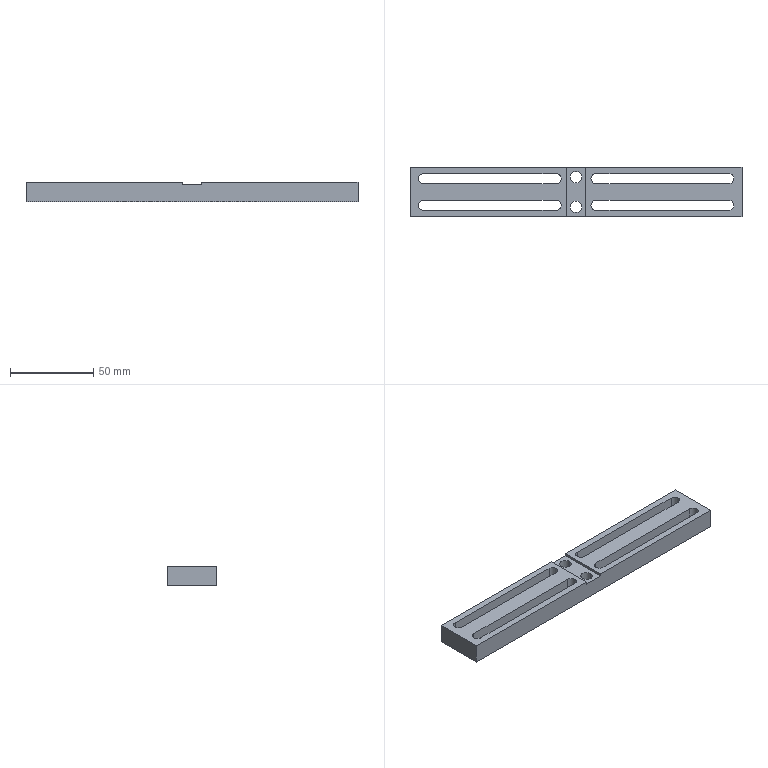Part | SolidWorks | features ICE 2, Extrusion 1 | 1 solid | 34 faces | box 200 x 30 x 12 mm | volume 46255 mm3 | plane 18 | cylinder 16 | commonest cylinder face diameters 6 x12 7 x4
STEP:
#1=CARTESIAN_POINT('',(-3.5,9.,0.));
#2=VERTEX_POINT('',#1);
#3=CARTESIAN_POINT('',(3.5,9.,0.));
#4=VERTEX_POINT('',#3);
#5=CARTESIAN_POINT('',(0.,9.,0.));
#6=DIRECTION('',(0.,0.,1.));
#7=DIRECTION('',(-1.,0.,0.));
#8=AXIS2_PLACEMENT_3D('',#5,#6,#7);
#9=CIRCLE('',#8,3.5);
#10=EDGE_CURVE('',#2,#4,#9,.T.);
#11=ORIENTED_EDGE('',*,*,#10,.F.);
#12=CARTESIAN_POINT('',(-3.5,9.,10.5));
#13=VERTEX_POINT('',#12);
#14=CARTESIAN_POINT('',(-3.5,9.,-0.001));
#15=DIRECTION('',(0.,0.,1.));
#16=VECTOR('',#15,1000.);
#17=LINE('',#14,#16);
#18=EDGE_CURVE('',#2,#13,#17,.T.);
#19=ORIENTED_EDGE('',*,*,#18,.T.);
#20=CARTESIAN_POINT('',(3.5,9.,10.5));
#21=VERTEX_POINT('',#20);
#22=CARTESIAN_POINT('',(0.,9.,10.5));
#23=DIRECTION('',(0.,0.,1.));
#24=DIRECTION('',(1.,0.,0.));
#25=AXIS2_PLACEMENT_3D('',#22,#23,#24);
#26=CIRCLE('',#25,3.5);
#27=EDGE_CURVE('',#13,#21,#26,.T.);
#28=ORIENTED_EDGE('',*,*,#27,.T.);
#29=CARTESIAN_POINT('',(3.5,9.,-0.001));
#30=DIRECTION('',(0.,0.,1.));
#31=VECTOR('',#30,1000.);
#32=LINE('',#29,#31);
#33=EDGE_CURVE('',#4,#21,#32,.T.);
#34=ORIENTED_EDGE('',*,*,#33,.F.);
#35=EDGE_LOOP('',(#11,#19,#28,#34));
#36=FACE_OUTER_BOUND('',#35,.T.);
#37=CARTESIAN_POINT('',(0.,9.,-0.001));
#38=DIRECTION('',(0.,0.,1.));
#39=DIRECTION('',(1.,0.,0.));
#40=AXIS2_PLACEMENT_3D('',#37,#38,#39);
#41=CYLINDRICAL_SURFACE('',#40,3.5);
#42=ADVANCED_FACE('',(#36),#41,.F.);
#43=CARTESIAN_POINT('',(-3.5,-9.,0.));
#44=VERTEX_POINT('',#43);
#45=CARTESIAN_POINT('',(3.5,-9.,0.));
#46=VERTEX_POINT('',#45);
#47=CARTESIAN_POINT('',(0.,-9.,0.));
#48=DIRECTION('',(0.,0.,1.));
#49=DIRECTION('',(-1.,0.,0.));
#50=AXIS2_PLACEMENT_3D('',#47,#48,#49);
#51=CIRCLE('',#50,3.5);
#52=EDGE_CURVE('',#44,#46,#51,.T.);
#53=ORIENTED_EDGE('',*,*,#52,.F.);
#54=CARTESIAN_POINT('',(-3.5,-9.,10.5));
#55=VERTEX_POINT('',#54);
#56=CARTESIAN_POINT('',(-3.5,-9.,-0.001));
#57=DIRECTION('',(0.,0.,1.));
#58=VECTOR('',#57,1000.);
#59=LINE('',#56,#58);
#60=EDGE_CURVE('',#44,#55,#59,.T.);
#61=ORIENTED_EDGE('',*,*,#60,.T.);
#62=CARTESIAN_POINT('',(3.5,-9.,10.5));
#63=VERTEX_POINT('',#62);
#64=CARTESIAN_POINT('',(0.,-9.,10.5));
#65=DIRECTION('',(0.,0.,1.));
#66=DIRECTION('',(1.,0.,0.));
#67=AXIS2_PLACEMENT_3D('',#64,#65,#66);
#68=CIRCLE('',#67,3.5);
#69=EDGE_CURVE('',#55,#63,#68,.T.);
#70=ORIENTED_EDGE('',*,*,#69,.T.);
#71=CARTESIAN_POINT('',(3.5,-9.,-0.001));
#72=DIRECTION('',(0.,0.,1.));
#73=VECTOR('',#72,1000.);
#74=LINE('',#71,#73);
#75=EDGE_CURVE('',#46,#63,#74,.T.);
#76=ORIENTED_EDGE('',*,*,#75,.F.);
#77=EDGE_LOOP('',(#53,#61,#70,#76));
#78=FACE_OUTER_BOUND('',#77,.T.);
#79=CARTESIAN_POINT('',(0.,-9.,-0.001));
#80=DIRECTION('',(0.,0.,1.));
#81=DIRECTION('',(1.,0.,0.));
#82=AXIS2_PLACEMENT_3D('',#79,#80,#81);
#83=CYLINDRICAL_SURFACE('',#82,3.5);
#84=ADVANCED_FACE('',(#78),#83,.F.);
#85=CARTESIAN_POINT('',(12.,-5.,12.));
#86=VERTEX_POINT('',#85);
#87=CARTESIAN_POINT('',(9.,-8.,12.));
#88=VERTEX_POINT('',#87);
#89=CARTESIAN_POINT('',(12.,-8.,12.));
#90=DIRECTION('',(0.,0.,1.));
#91=DIRECTION('',(1.,0.,0.));
#92=AXIS2_PLACEMENT_3D('',#89,#90,#91);
#93=CIRCLE('',#92,3.);
#94=EDGE_CURVE('',#86,#88,#93,.T.);
#95=ORIENTED_EDGE('',*,*,#94,.T.);
#96=CARTESIAN_POINT('',(9.,-8.,0.));
#97=VERTEX_POINT('',#96);
#98=CARTESIAN_POINT('',(9.,-8.,12.));
#99=DIRECTION('',(0.,0.,-1.));
#100=VECTOR('',#99,1000.);
#101=LINE('',#98,#100);
#102=EDGE_CURVE('',#88,#97,#101,.T.);
#103=ORIENTED_EDGE('',*,*,#102,.T.);
#104=CARTESIAN_POINT('',(12.,-5.,0.));
#105=VERTEX_POINT('',#104);
#106=CARTESIAN_POINT('',(12.,-8.,0.));
#107=DIRECTION('',(0.,0.,1.));
#108=DIRECTION('',(1.,0.,0.));
#109=AXIS2_PLACEMENT_3D('',#106,#107,#108);
#110=CIRCLE('',#109,3.);
#111=EDGE_CURVE('',#105,#97,#110,.T.);
#112=ORIENTED_EDGE('',*,*,#111,.F.);
#113=CARTESIAN_POINT('',(12.,-5.,12.));
#114=DIRECTION('',(0.,0.,-1.));
#115=VECTOR('',#114,1000.);
#116=LINE('',#113,#115);
#117=EDGE_CURVE('',#86,#105,#116,.T.);
#118=ORIENTED_EDGE('',*,*,#117,.F.);
#119=EDGE_LOOP('',(#95,#103,#112,#118));
#120=FACE_OUTER_BOUND('',#119,.T.);
#121=CARTESIAN_POINT('',(12.,-8.,12.));
#122=DIRECTION('',(0.,0.,-1.));
#123=DIRECTION('',(-1.,0.,0.));
#124=AXIS2_PLACEMENT_3D('',#121,#122,#123);
#125=CYLINDRICAL_SURFACE('',#124,3.);
#126=ADVANCED_FACE('',(#120),#125,.F.);
#127=CARTESIAN_POINT('',(12.,11.,12.));
#128=VERTEX_POINT('',#127);
#129=CARTESIAN_POINT('',(9.,8.,12.));
#130=VERTEX_POINT('',#129);
#131=CARTESIAN_POINT('',(12.,8.,12.));
#132=DIRECTION('',(0.,0.,1.));
#133=DIRECTION('',(-1.,0.,0.));
#134=AXIS2_PLACEMENT_3D('',#131,#132,#133);
#135=CIRCLE('',#134,3.);
#136=EDGE_CURVE('',#128,#130,#135,.T.);
#137=ORIENTED_EDGE('',*,*,#136,.T.);
#138=CARTESIAN_POINT('',(9.,8.,0.));
#139=VERTEX_POINT('',#138);
#140=CARTESIAN_POINT('',(9.,8.,12.));
#141=DIRECTION('',(0.,0.,-1.));
#142=VECTOR('',#141,1000.);
#143=LINE('',#140,#142);
#144=EDGE_CURVE('',#130,#139,#143,.T.);
#145=ORIENTED_EDGE('',*,*,#144,.T.);
#146=CARTESIAN_POINT('',(12.,11.,0.));
#147=VERTEX_POINT('',#146);
#148=CARTESIAN_POINT('',(12.,8.,0.));
#149=DIRECTION('',(0.,0.,1.));
#150=DIRECTION('',(-1.,0.,0.));
#151=AXIS2_PLACEMENT_3D('',#148,#149,#150);
#152=CIRCLE('',#151,3.);
#153=EDGE_CURVE('',#147,#139,#152,.T.);
#154=ORIENTED_EDGE('',*,*,#153,.F.);
#155=CARTESIAN_POINT('',(12.,11.,12.));
#156=DIRECTION('',(0.,0.,-1.));
#157=VECTOR('',#156,1000.);
#158=LINE('',#155,#157);
#159=EDGE_CURVE('',#128,#147,#158,.T.);
#160=ORIENTED_EDGE('',*,*,#159,.F.);
#161=EDGE_LOOP('',(#137,#145,#154,#160));
#162=FACE_OUTER_BOUND('',#161,.T.);
#163=CARTESIAN_POINT('',(12.,8.,12.));
#164=DIRECTION('',(0.,0.,-1.));
#165=DIRECTION('',(-1.,0.,0.));
#166=AXIS2_PLACEMENT_3D('',#163,#164,#165);
#167=CYLINDRICAL_SURFACE('',#166,3.);
#168=ADVANCED_FACE('',(#162),#167,.F.);
#169=CARTESIAN_POINT('',(-92.,-5.,12.));
#170=VERTEX_POINT('',#169);
#171=CARTESIAN_POINT('',(-95.,-8.,12.));
#172=VERTEX_POINT('',#171);
#173=CARTESIAN_POINT('',(-92.,-8.,12.));
#174=DIRECTION('',(0.,0.,1.));
#175=DIRECTION('',(-1.,0.,0.));
#176=AXIS2_PLACEMENT_3D('',#173,#174,#175);
#177=CIRCLE('',#176,3.);
#178=EDGE_CURVE('',#170,#172,#177,.T.);
#179=ORIENTED_EDGE('',*,*,#178,.T.);
#180=CARTESIAN_POINT('',(-95.,-8.,0.));
#181=VERTEX_POINT('',#180);
#182=CARTESIAN_POINT('',(-95.,-8.,12.));
#183=DIRECTION('',(0.,0.,-1.));
#184=VECTOR('',#183,1000.);
#185=LINE('',#182,#184);
#186=EDGE_CURVE('',#172,#181,#185,.T.);
#187=ORIENTED_EDGE('',*,*,#186,.T.);
#188=CARTESIAN_POINT('',(-92.,-5.,0.));
#189=VERTEX_POINT('',#188);
#190=CARTESIAN_POINT('',(-92.,-8.,0.));
#191=DIRECTION('',(0.,0.,1.));
#192=DIRECTION('',(-1.,0.,0.));
#193=AXIS2_PLACEMENT_3D('',#190,#191,#192);
#194=CIRCLE('',#193,3.);
#195=EDGE_CURVE('',#189,#181,#194,.T.);
#196=ORIENTED_EDGE('',*,*,#195,.F.);
#197=CARTESIAN_POINT('',(-92.,-5.,12.));
#198=DIRECTION('',(0.,0.,-1.));
#199=VECTOR('',#198,1000.);
#200=LINE('',#197,#199);
#201=EDGE_CURVE('',#170,#189,#200,.T.);
#202=ORIENTED_EDGE('',*,*,#201,.F.);
#203=EDGE_LOOP('',(#179,#187,#196,#202));
#204=FACE_OUTER_BOUND('',#203,.T.);
#205=CARTESIAN_POINT('',(-92.,-8.,12.));
#206=DIRECTION('',(0.,0.,-1.));
#207=DIRECTION('',(-1.,0.,0.));
#208=AXIS2_PLACEMENT_3D('',#205,#206,#207);
#209=CYLINDRICAL_SURFACE('',#208,3.);
#210=ADVANCED_FACE('',(#204),#209,.F.);
#211=CARTESIAN_POINT('',(-92.,11.,12.));
#212=VERTEX_POINT('',#211);
#213=CARTESIAN_POINT('',(-95.,8.,12.));
#214=VERTEX_POINT('',#213);
#215=CARTESIAN_POINT('',(-92.,8.,12.));
#216=DIRECTION('',(0.,0.,1.));
#217=DIRECTION('',(1.,0.,0.));
#218=AXIS2_PLACEMENT_3D('',#215,#216,#217);
#219=CIRCLE('',#218,3.);
#220=EDGE_CURVE('',#212,#214,#219,.T.);
#221=ORIENTED_EDGE('',*,*,#220,.T.);
#222=CARTESIAN_POINT('',(-95.,8.,0.));
#223=VERTEX_POINT('',#222);
#224=CARTESIAN_POINT('',(-95.,8.,12.));
#225=DIRECTION('',(0.,0.,-1.));
#226=VECTOR('',#225,1000.);
#227=LINE('',#224,#226);
#228=EDGE_CURVE('',#214,#223,#227,.T.);
#229=ORIENTED_EDGE('',*,*,#228,.T.);
#230=CARTESIAN_POINT('',(-92.,11.,0.));
#231=VERTEX_POINT('',#230);
#232=CARTESIAN_POINT('',(-92.,8.,0.));
#233=DIRECTION('',(0.,0.,1.));
#234=DIRECTION('',(1.,0.,0.));
#235=AXIS2_PLACEMENT_3D('',#232,#233,#234);
#236=CIRCLE('',#235,3.);
#237=EDGE_CURVE('',#231,#223,#236,.T.);
#238=ORIENTED_EDGE('',*,*,#237,.F.);
#239=CARTESIAN_POINT('',(-92.,11.,12.));
#240=DIRECTION('',(0.,0.,-1.));
#241=VECTOR('',#240,1000.);
#242=LINE('',#239,#241);
#243=EDGE_CURVE('',#212,#231,#242,.T.);
#244=ORIENTED_EDGE('',*,*,#243,.F.);
#245=EDGE_LOOP('',(#221,#229,#238,#244));
#246=FACE_OUTER_BOUND('',#245,.T.);
#247=CARTESIAN_POINT('',(-92.,8.,12.));
#248=DIRECTION('',(0.,0.,-1.));
#249=DIRECTION('',(-1.,0.,0.));
#250=AXIS2_PLACEMENT_3D('',#247,#248,#249);
#251=CYLINDRICAL_SURFACE('',#250,3.);
#252=ADVANCED_FACE('',(#246),#251,.F.);
#253=CARTESIAN_POINT('',(92.,-11.,12.));
#254=VERTEX_POINT('',#253);
#255=CARTESIAN_POINT('',(92.,-5.,12.));
#256=VERTEX_POINT('',#255);
#257=CARTESIAN_POINT('',(92.,-8.,12.));
#258=DIRECTION('',(0.,0.,1.));
#259=DIRECTION('',(1.,0.,0.));
#260=AXIS2_PLACEMENT_3D('',#257,#258,#259);
#261=CIRCLE('',#260,3.);
#262=EDGE_CURVE('',#254,#256,#261,.T.);
#263=ORIENTED_EDGE('',*,*,#262,.F.);
#264=CARTESIAN_POINT('',(12.,-11.,12.));
#265=VERTEX_POINT('',#264);
#266=CARTESIAN_POINT('',(92.,-11.,12.));
#267=DIRECTION('',(1.,0.,0.));
#268=VECTOR('',#267,1000.);
#269=LINE('',#266,#268);
#270=EDGE_CURVE('',#265,#254,#269,.T.);
#271=ORIENTED_EDGE('',*,*,#270,.F.);
#272=CARTESIAN_POINT('',(12.,-8.,12.));
#273=DIRECTION('',(0.,0.,1.));
#274=DIRECTION('',(1.,0.,0.));
#275=AXIS2_PLACEMENT_3D('',#272,#273,#274);
#276=CIRCLE('',#275,3.);
#277=EDGE_CURVE('',#88,#265,#276,.T.);
#278=ORIENTED_EDGE('',*,*,#277,.F.);
#279=ORIENTED_EDGE('',*,*,#94,.F.);
#280=CARTESIAN_POINT('',(92.,-5.,12.));
#281=DIRECTION('',(-1.,0.,0.));
#282=VECTOR('',#281,1000.);
#283=LINE('',#280,#282);
#284=EDGE_CURVE('',#256,#86,#283,.T.);
#285=ORIENTED_EDGE('',*,*,#284,.F.);
#286=EDGE_LOOP('',(#263,#271,#278,#279,#285));
#287=FACE_BOUND('',#286,.T.);
#288=CARTESIAN_POINT('',(92.,5.,12.));
#289=VERTEX_POINT('',#288);
#290=CARTESIAN_POINT('',(92.,11.,12.));
#291=VERTEX_POINT('',#290);
#292=CARTESIAN_POINT('',(92.,8.,12.));
#293=DIRECTION('',(0.,0.,1.));
#294=DIRECTION('',(-1.,0.,0.));
#295=AXIS2_PLACEMENT_3D('',#292,#293,#294);
#296=CIRCLE('',#295,3.);
#297=EDGE_CURVE('',#289,#291,#296,.T.);
#298=ORIENTED_EDGE('',*,*,#297,.F.);
#299=CARTESIAN_POINT('',(12.,5.,12.));
#300=VERTEX_POINT('',#299);
#301=CARTESIAN_POINT('',(92.,5.,12.));
#302=DIRECTION('',(1.,0.,0.));
#303=VECTOR('',#302,1000.);
#304=LINE('',#301,#303);
#305=EDGE_CURVE('',#300,#289,#304,.T.);
#306=ORIENTED_EDGE('',*,*,#305,.F.);
#307=CARTESIAN_POINT('',(12.,8.,12.));
#308=DIRECTION('',(0.,0.,1.));
#309=DIRECTION('',(-1.,0.,0.));
#310=AXIS2_PLACEMENT_3D('',#307,#308,#309);
#311=CIRCLE('',#310,3.);
#312=EDGE_CURVE('',#130,#300,#311,.T.);
#313=ORIENTED_EDGE('',*,*,#312,.F.);
#314=ORIENTED_EDGE('',*,*,#136,.F.);
#315=CARTESIAN_POINT('',(92.,11.,12.));
#316=DIRECTION('',(-1.,0.,0.));
#317=VECTOR('',#316,1000.);
#318=LINE('',#315,#317);
#319=EDGE_CURVE('',#291,#128,#318,.T.);
#320=ORIENTED_EDGE('',*,*,#319,.F.);
#321=EDGE_LOOP('',(#298,#306,#313,#314,#320));
#322=FACE_BOUND('',#321,.T.);
#323=CARTESIAN_POINT('',(100.,15.,12.));
#324=VERTEX_POINT('',#323);
#325=CARTESIAN_POINT('',(6.,15.,12.));
#326=VERTEX_POINT('',#325);
#327=CARTESIAN_POINT('',(-100.,15.,12.));
#328=DIRECTION('',(-1.,0.,0.));
#329=VECTOR('',#328,1000.);
#330=LINE('',#327,#329);
#331=EDGE_CURVE('',#324,#326,#330,.T.);
#332=ORIENTED_EDGE('',*,*,#331,.T.);
#333=CARTESIAN_POINT('',(6.,-15.,12.));
#334=VERTEX_POINT('',#333);
#335=CARTESIAN_POINT('',(6.,-15.,12.));
#336=DIRECTION('',(0.,1.,0.));
#337=VECTOR('',#336,1000.);
#338=LINE('',#335,#337);
#339=EDGE_CURVE('',#334,#326,#338,.T.);
#340=ORIENTED_EDGE('',*,*,#339,.F.);
#341=CARTESIAN_POINT('',(100.,-15.,12.));
#342=VERTEX_POINT('',#341);
#343=CARTESIAN_POINT('',(-100.,-15.,12.));
#344=DIRECTION('',(1.,0.,0.));
#345=VECTOR('',#344,1000.);
#346=LINE('',#343,#345);
#347=EDGE_CURVE('',#334,#342,#346,.T.);
#348=ORIENTED_EDGE('',*,*,#347,.T.);
#349=CARTESIAN_POINT('',(100.,-15.,12.));
#350=DIRECTION('',(0.,1.,0.));
#351=VECTOR('',#350,1000.);
#352=LINE('',#349,#351);
#353=EDGE_CURVE('',#342,#324,#352,.T.);
#354=ORIENTED_EDGE('',*,*,#353,.T.);
#355=EDGE_LOOP('',(#332,#340,#348,#354));
#356=FACE_OUTER_BOUND('',#355,.T.);
#357=CARTESIAN_POINT('',(0.,0.,12.));
#358=DIRECTION('',(0.,0.,-1.));
#359=DIRECTION('',(-1.,0.,0.));
#360=AXIS2_PLACEMENT_3D('',#357,#358,#359);
#361=PLANE('',#360);
#362=ADVANCED_FACE('',(#287,#322,#356),#361,.F.);
#363=ORIENTED_EDGE('',*,*,#220,.F.);
#364=CARTESIAN_POINT('',(-12.,11.,12.));
#365=VERTEX_POINT('',#364);
#366=CARTESIAN_POINT('',(-92.,11.,12.));
#367=DIRECTION('',(-1.,0.,0.));
#368=VECTOR('',#367,1000.);
#369=LINE('',#366,#368);
#370=EDGE_CURVE('',#365,#212,#369,.T.);
#371=ORIENTED_EDGE('',*,*,#370,.F.);
#372=CARTESIAN_POINT('',(-12.,5.,12.));
#373=VERTEX_POINT('',#372);
#374=CARTESIAN_POINT('',(-12.,8.,12.));
#375=DIRECTION('',(0.,0.,1.));
#376=DIRECTION('',(1.,0.,0.));
#377=AXIS2_PLACEMENT_3D('',#374,#375,#376);
#378=CIRCLE('',#377,3.);
#379=EDGE_CURVE('',#373,#365,#378,.T.);
#380=ORIENTED_EDGE('',*,*,#379,.F.);
#381=CARTESIAN_POINT('',(-92.,5.,12.));
#382=VERTEX_POINT('',#381);
#383=CARTESIAN_POINT('',(-92.,5.,12.));
#384=DIRECTION('',(1.,0.,0.));
#385=VECTOR('',#384,1000.);
#386=LINE('',#383,#385);
#387=EDGE_CURVE('',#382,#373,#386,.T.);
#388=ORIENTED_EDGE('',*,*,#387,.F.);
#389=CARTESIAN_POINT('',(-92.,8.,12.));
#390=DIRECTION('',(0.,0.,1.));
#391=DIRECTION('',(1.,0.,0.));
#392=AXIS2_PLACEMENT_3D('',#389,#390,#391);
#393=CIRCLE('',#392,3.);
#394=EDGE_CURVE('',#214,#382,#393,.T.);
#395=ORIENTED_EDGE('',*,*,#394,.F.);
#396=EDGE_LOOP('',(#363,#371,#380,#388,#395));
#397=FACE_BOUND('',#396,.T.);
#398=CARTESIAN_POINT('',(-100.,-15.,12.));
#399=VERTEX_POINT('',#398);
#400=CARTESIAN_POINT('',(-6.,-15.,12.));
#401=VERTEX_POINT('',#400);
#402=CARTESIAN_POINT('',(-100.,-15.,12.));
#403=DIRECTION('',(1.,0.,0.));
#404=VECTOR('',#403,1000.);
#405=LINE('',#402,#404);
#406=EDGE_CURVE('',#399,#401,#405,.T.);
#407=ORIENTED_EDGE('',*,*,#406,.T.);
#408=CARTESIAN_POINT('',(-6.,15.,12.));
#409=VERTEX_POINT('',#408);
#410=CARTESIAN_POINT('',(-6.,-15.,12.));
#411=DIRECTION('',(0.,-1.,0.));
#412=VECTOR('',#411,1000.);
#413=LINE('',#410,#412);
#414=EDGE_CURVE('',#409,#401,#413,.T.);
#415=ORIENTED_EDGE('',*,*,#414,.F.);
#416=CARTESIAN_POINT('',(-100.,15.,12.));
#417=VERTEX_POINT('',#416);
#418=CARTESIAN_POINT('',(-100.,15.,12.));
#419=DIRECTION('',(-1.,0.,0.));
#420=VECTOR('',#419,1000.);
#421=LINE('',#418,#420);
#422=EDGE_CURVE('',#409,#417,#421,.T.);
#423=ORIENTED_EDGE('',*,*,#422,.T.);
#424=CARTESIAN_POINT('',(-100.,-15.,12.));
#425=DIRECTION('',(0.,-1.,0.));
#426=VECTOR('',#425,1000.);
#427=LINE('',#424,#426);
#428=EDGE_CURVE('',#417,#399,#427,.T.);
#429=ORIENTED_EDGE('',*,*,#428,.T.);
#430=EDGE_LOOP('',(#407,#415,#423,#429));
#431=FACE_OUTER_BOUND('',#430,.T.);
#432=ORIENTED_EDGE('',*,*,#178,.F.);
#433=CARTESIAN_POINT('',(-12.,-5.,12.));
#434=VERTEX_POINT('',#433);
#435=CARTESIAN_POINT('',(-92.,-5.,12.));
#436=DIRECTION('',(-1.,0.,0.));
#437=VECTOR('',#436,1000.);
#438=LINE('',#435,#437);
#439=EDGE_CURVE('',#434,#170,#438,.T.);
#440=ORIENTED_EDGE('',*,*,#439,.F.);
#441=CARTESIAN_POINT('',(-12.,-11.,12.));
#442=VERTEX_POINT('',#441);
#443=CARTESIAN_POINT('',(-12.,-8.,12.));
#444=DIRECTION('',(0.,0.,1.));
#445=DIRECTION('',(-1.,0.,0.));
#446=AXIS2_PLACEMENT_3D('',#443,#444,#445);
#447=CIRCLE('',#446,3.);
#448=EDGE_CURVE('',#442,#434,#447,.T.);
#449=ORIENTED_EDGE('',*,*,#448,.F.);
#450=CARTESIAN_POINT('',(-92.,-11.,12.));
#451=VERTEX_POINT('',#450);
#452=CARTESIAN_POINT('',(-92.,-11.,12.));
#453=DIRECTION('',(1.,0.,0.));
#454=VECTOR('',#453,1000.);
#455=LINE('',#452,#454);
#456=EDGE_CURVE('',#451,#442,#455,.T.);
#457=ORIENTED_EDGE('',*,*,#456,.F.);
#458=CARTESIAN_POINT('',(-92.,-8.,12.));
#459=DIRECTION('',(0.,0.,1.));
#460=DIRECTION('',(-1.,0.,0.));
#461=AXIS2_PLACEMENT_3D('',#458,#459,#460);
#462=CIRCLE('',#461,3.);
#463=EDGE_CURVE('',#172,#451,#462,.T.);
#464=ORIENTED_EDGE('',*,*,#463,.F.);
#465=EDGE_LOOP('',(#432,#440,#449,#457,#464));
#466=FACE_BOUND('',#465,.T.);
#467=CARTESIAN_POINT('',(0.,0.,12.));
#468=DIRECTION('',(0.,0.,-1.));
#469=DIRECTION('',(-1.,0.,0.));
#470=AXIS2_PLACEMENT_3D('',#467,#468,#469);
#471=PLANE('',#470);
#472=ADVANCED_FACE('',(#397,#431,#466),#471,.F.);
#473=CARTESIAN_POINT('',(0.,9.,0.));
#474=DIRECTION('',(0.,0.,1.));
#475=DIRECTION('',(-1.,0.,0.));
#476=AXIS2_PLACEMENT_3D('',#473,#474,#475);
#477=CIRCLE('',#476,3.5);
#478=EDGE_CURVE('',#4,#2,#477,.T.);
#479=ORIENTED_EDGE('',*,*,#478,.T.);
#480=ORIENTED_EDGE('',*,*,#10,.T.);
#481=EDGE_LOOP('',(#479,#480));
#482=FACE_BOUND('',#481,.T.);
#483=CARTESIAN_POINT('',(0.,-9.,0.));
#484=DIRECTION('',(0.,0.,1.));
#485=DIRECTION('',(-1.,0.,0.));
#486=AXIS2_PLACEMENT_3D('',#483,#484,#485);
#487=CIRCLE('',#486,3.5);
#488=EDGE_CURVE('',#46,#44,#487,.T.);
#489=ORIENTED_EDGE('',*,*,#488,.T.);
#490=ORIENTED_EDGE('',*,*,#52,.T.);
#491=EDGE_LOOP('',(#489,#490));
#492=FACE_BOUND('',#491,.T.);
#493=CARTESIAN_POINT('',(100.,-15.,0.));
#494=VERTEX_POINT('',#493);
#495=CARTESIAN_POINT('',(100.,15.,0.));
#496=VERTEX_POINT('',#495);
#497=CARTESIAN_POINT('',(100.,-15.,0.));
#498=DIRECTION('',(0.,1.,0.));
#499=VECTOR('',#498,1000.);
#500=LINE('',#497,#499);
#501=EDGE_CURVE('',#494,#496,#500,.T.);
#502=ORIENTED_EDGE('',*,*,#501,.F.);
#503=CARTESIAN_POINT('',(-100.,-15.,0.));
#504=VERTEX_POINT('',#503);
#505=CARTESIAN_POINT('',(-100.,-15.,0.));
#506=DIRECTION('',(1.,0.,0.));
#507=VECTOR('',#506,1000.);
#508=LINE('',#505,#507);
#509=EDGE_CURVE('',#504,#494,#508,.T.);
#510=ORIENTED_EDGE('',*,*,#509,.F.);
#511=CARTESIAN_POINT('',(-100.,15.,0.));
#512=VERTEX_POINT('',#511);
#513=CARTESIAN_POINT('',(-100.,-15.,0.));
#514=DIRECTION('',(0.,-1.,0.));
#515=VECTOR('',#514,1000.);
#516=LINE('',#513,#515);
#517=EDGE_CURVE('',#512,#504,#516,.T.);
#518=ORIENTED_EDGE('',*,*,#517,.F.);
#519=CARTESIAN_POINT('',(-100.,15.,0.));
#520=DIRECTION('',(-1.,0.,0.));
#521=VECTOR('',#520,1000.);
#522=LINE('',#519,#521);
#523=EDGE_CURVE('',#496,#512,#522,.T.);
#524=ORIENTED_EDGE('',*,*,#523,.F.);
#525=EDGE_LOOP('',(#502,#510,#518,#524));
#526=FACE_OUTER_BOUND('',#525,.T.);
#527=CARTESIAN_POINT('',(-12.,11.,0.));
#528=VERTEX_POINT('',#527);
#529=CARTESIAN_POINT('',(-92.,11.,0.));
#530=DIRECTION('',(-1.,0.,0.));
#531=VECTOR('',#530,1000.);
#532=LINE('',#529,#531);
#533=EDGE_CURVE('',#528,#231,#532,.T.);
#534=ORIENTED_EDGE('',*,*,#533,.T.);
#535=ORIENTED_EDGE('',*,*,#237,.T.);
#536=CARTESIAN_POINT('',(-92.,5.,0.));
#537=VERTEX_POINT('',#536);
#538=CARTESIAN_POINT('',(-92.,8.,0.));
#539=DIRECTION('',(0.,0.,1.));
#540=DIRECTION('',(1.,0.,0.));
#541=AXIS2_PLACEMENT_3D('',#538,#539,#540);
#542=CIRCLE('',#541,3.);
#543=EDGE_CURVE('',#223,#537,#542,.T.);
#544=ORIENTED_EDGE('',*,*,#543,.T.);
#545=CARTESIAN_POINT('',(-12.,5.,0.));
#546=VERTEX_POINT('',#545);
#547=CARTESIAN_POINT('',(-92.,5.,0.));
#548=DIRECTION('',(1.,0.,0.));
#549=VECTOR('',#548,1000.);
#550=LINE('',#547,#549);
#551=EDGE_CURVE('',#537,#546,#550,.T.);
#552=ORIENTED_EDGE('',*,*,#551,.T.);
#553=CARTESIAN_POINT('',(-12.,8.,0.));
#554=DIRECTION('',(0.,0.,1.));
#555=DIRECTION('',(1.,0.,0.));
#556=AXIS2_PLACEMENT_3D('',#553,#554,#555);
#557=CIRCLE('',#556,3.);
#558=EDGE_CURVE('',#546,#528,#557,.T.);
#559=ORIENTED_EDGE('',*,*,#558,.T.);
#560=EDGE_LOOP('',(#534,#535,#544,#552,#559));
#561=FACE_BOUND('',#560,.T.);
#562=CARTESIAN_POINT('',(-12.,-5.,0.));
#563=VERTEX_POINT('',#562);
#564=CARTESIAN_POINT('',(-92.,-5.,0.));
#565=DIRECTION('',(-1.,0.,0.));
#566=VECTOR('',#565,1000.);
#567=LINE('',#564,#566);
#568=EDGE_CURVE('',#563,#189,#567,.T.);
#569=ORIENTED_EDGE('',*,*,#568,.T.);
#570=ORIENTED_EDGE('',*,*,#195,.T.);
#571=CARTESIAN_POINT('',(-92.,-11.,0.));
#572=VERTEX_POINT('',#571);
#573=CARTESIAN_POINT('',(-92.,-8.,0.));
#574=DIRECTION('',(0.,0.,1.));
#575=DIRECTION('',(-1.,0.,0.));
#576=AXIS2_PLACEMENT_3D('',#573,#574,#575);
#577=CIRCLE('',#576,3.);
#578=EDGE_CURVE('',#181,#572,#577,.T.);
#579=ORIENTED_EDGE('',*,*,#578,.T.);
#580=CARTESIAN_POINT('',(-12.,-11.,0.));
#581=VERTEX_POINT('',#580);
#582=CARTESIAN_POINT('',(-92.,-11.,0.));
#583=DIRECTION('',(1.,0.,0.));
#584=VECTOR('',#583,1000.);
#585=LINE('',#582,#584);
#586=EDGE_CURVE('',#572,#581,#585,.T.);
#587=ORIENTED_EDGE('',*,*,#586,.T.);
#588=CARTESIAN_POINT('',(-12.,-8.,0.));
#589=DIRECTION('',(0.,0.,1.));
#590=DIRECTION('',(-1.,0.,0.));
#591=AXIS2_PLACEMENT_3D('',#588,#589,#590);
#592=CIRCLE('',#591,3.);
#593=EDGE_CURVE('',#581,#563,#592,.T.);
#594=ORIENTED_EDGE('',*,*,#593,.T.);
#595=EDGE_LOOP('',(#569,#570,#579,#587,#594));
#596=FACE_BOUND('',#595,.T.);
#597=CARTESIAN_POINT('',(12.,5.,0.));
#598=VERTEX_POINT('',#597);
#599=CARTESIAN_POINT('',(92.,5.,0.));
#600=VERTEX_POINT('',#599);
#601=CARTESIAN_POINT('',(92.,5.,0.));
#602=DIRECTION('',(1.,0.,0.));
#603=VECTOR('',#602,1000.);
#604=LINE('',#601,#603);
#605=EDGE_CURVE('',#598,#600,#604,.T.);
#606=ORIENTED_EDGE('',*,*,#605,.T.);
#607=CARTESIAN_POINT('',(92.,11.,0.));
#608=VERTEX_POINT('',#607);
#609=CARTESIAN_POINT('',(92.,8.,0.));
#610=DIRECTION('',(0.,0.,1.));
#611=DIRECTION('',(-1.,0.,0.));
#612=AXIS2_PLACEMENT_3D('',#609,#610,#611);
#613=CIRCLE('',#612,3.);
#614=EDGE_CURVE('',#600,#608,#613,.T.);
#615=ORIENTED_EDGE('',*,*,#614,.T.);
#616=CARTESIAN_POINT('',(92.,11.,0.));
#617=DIRECTION('',(-1.,0.,0.));
#618=VECTOR('',#617,1000.);
#619=LINE('',#616,#618);
#620=EDGE_CURVE('',#608,#147,#619,.T.);
#621=ORIENTED_EDGE('',*,*,#620,.T.);
#622=ORIENTED_EDGE('',*,*,#153,.T.);
#623=CARTESIAN_POINT('',(12.,8.,0.));
#624=DIRECTION('',(0.,0.,1.));
#625=DIRECTION('',(-1.,0.,0.));
#626=AXIS2_PLACEMENT_3D('',#623,#624,#625);
#627=CIRCLE('',#626,3.);
#628=EDGE_CURVE('',#139,#598,#627,.T.);
#629=ORIENTED_EDGE('',*,*,#628,.T.);
#630=EDGE_LOOP('',(#606,#615,#621,#622,#629));
#631=FACE_BOUND('',#630,.T.);
#632=CARTESIAN_POINT('',(12.,-11.,0.));
#633=VERTEX_POINT('',#632);
#634=CARTESIAN_POINT('',(92.,-11.,0.));
#635=VERTEX_POINT('',#634);
#636=CARTESIAN_POINT('',(92.,-11.,0.));
#637=DIRECTION('',(1.,0.,0.));
#638=VECTOR('',#637,1000.);
#639=LINE('',#636,#638);
#640=EDGE_CURVE('',#633,#635,#639,.T.);
#641=ORIENTED_EDGE('',*,*,#640,.T.);
#642=CARTESIAN_POINT('',(92.,-5.,0.));
#643=VERTEX_POINT('',#642);
#644=CARTESIAN_POINT('',(92.,-8.,0.));
#645=DIRECTION('',(0.,0.,1.));
#646=DIRECTION('',(1.,0.,0.));
#647=AXIS2_PLACEMENT_3D('',#644,#645,#646);
#648=CIRCLE('',#647,3.);
#649=EDGE_CURVE('',#635,#643,#648,.T.);
#650=ORIENTED_EDGE('',*,*,#649,.T.);
#651=CARTESIAN_POINT('',(92.,-5.,0.));
#652=DIRECTION('',(-1.,0.,0.));
#653=VECTOR('',#652,1000.);
#654=LINE('',#651,#653);
#655=EDGE_CURVE('',#643,#105,#654,.T.);
#656=ORIENTED_EDGE('',*,*,#655,.T.);
#657=ORIENTED_EDGE('',*,*,#111,.T.);
#658=CARTESIAN_POINT('',(12.,-8.,0.));
#659=DIRECTION('',(0.,0.,1.));
#660=DIRECTION('',(1.,0.,0.));
#661=AXIS2_PLACEMENT_3D('',#658,#659,#660);
#662=CIRCLE('',#661,3.);
#663=EDGE_CURVE('',#97,#633,#662,.T.);
#664=ORIENTED_EDGE('',*,*,#663,.T.);
#665=EDGE_LOOP('',(#641,#650,#656,#657,#664));
#666=FACE_BOUND('',#665,.T.);
#667=CARTESIAN_POINT('',(0.,0.,0.));
#668=DIRECTION('',(0.,0.,-1.));
#669=DIRECTION('',(-1.,0.,0.));
#670=AXIS2_PLACEMENT_3D('',#667,#668,#669);
#671=PLANE('',#670);
#672=ADVANCED_FACE('',(#482,#492,#526,#561,#596,#631,#666),#671,.T.);
#673=ORIENTED_EDGE('',*,*,#501,.T.);
#674=CARTESIAN_POINT('',(100.,15.,12.));
#675=DIRECTION('',(0.,0.,-1.));
#676=VECTOR('',#675,1000.);
#677=LINE('',#674,#676);
#678=EDGE_CURVE('',#324,#496,#677,.T.);
#679=ORIENTED_EDGE('',*,*,#678,.F.);
#680=ORIENTED_EDGE('',*,*,#353,.F.);
#681=CARTESIAN_POINT('',(100.,-15.,12.));
#682=DIRECTION('',(0.,0.,-1.));
#683=VECTOR('',#682,1000.);
#684=LINE('',#681,#683);
#685=EDGE_CURVE('',#342,#494,#684,.T.);
#686=ORIENTED_EDGE('',*,*,#685,.T.);
#687=EDGE_LOOP('',(#673,#679,#680,#686));
#688=FACE_OUTER_BOUND('',#687,.T.);
#689=CARTESIAN_POINT('',(100.,-15.,12.));
#690=DIRECTION('',(-1.,0.,0.));
#691=DIRECTION('',(0.,0.,1.));
#692=AXIS2_PLACEMENT_3D('',#689,#690,#691);
#693=PLANE('',#692);
#694=ADVANCED_FACE('',(#688),#693,.F.);
#695=CARTESIAN_POINT('',(6.,15.,10.5));
#696=VERTEX_POINT('',#695);
#697=CARTESIAN_POINT('',(-6.,15.,10.5));
#698=VERTEX_POINT('',#697);
#699=CARTESIAN_POINT('',(-6.,15.,10.5));
#700=DIRECTION('',(-1.,0.,0.));
#701=VECTOR('',#700,1000.);
#702=LINE('',#699,#701);
#703=EDGE_CURVE('',#696,#698,#702,.T.);
#704=ORIENTED_EDGE('',*,*,#703,.F.);
#705=CARTESIAN_POINT('',(6.,15.,10.5));
#706=DIRECTION('',(0.,0.,1.));
#707=VECTOR('',#706,1000.);
#708=LINE('',#705,#707);
#709=EDGE_CURVE('',#696,#326,#708,.T.);
#710=ORIENTED_EDGE('',*,*,#709,.T.);
#711=ORIENTED_EDGE('',*,*,#331,.F.);
#712=ORIENTED_EDGE('',*,*,#678,.T.);
#713=ORIENTED_EDGE('',*,*,#523,.T.);
#714=CARTESIAN_POINT('',(-100.,15.,12.));
#715=DIRECTION('',(0.,0.,-1.));
#716=VECTOR('',#715,1000.);
#717=LINE('',#714,#716);
#718=EDGE_CURVE('',#417,#512,#717,.T.);
#719=ORIENTED_EDGE('',*,*,#718,.F.);
#720=ORIENTED_EDGE('',*,*,#422,.F.);
#721=CARTESIAN_POINT('',(-6.,15.,10.5));
#722=DIRECTION('',(0.,0.,1.));
#723=VECTOR('',#722,1000.);
#724=LINE('',#721,#723);
#725=EDGE_CURVE('',#698,#409,#724,.T.);
#726=ORIENTED_EDGE('',*,*,#725,.F.);
#727=EDGE_LOOP('',(#704,#710,#711,#712,#713,#719,#720,#726));
#728=FACE_OUTER_BOUND('',#727,.T.);
#729=CARTESIAN_POINT('',(-100.,15.,12.));
#730=DIRECTION('',(0.,-1.,0.));
#731=DIRECTION('',(0.,0.,-1.));
#732=AXIS2_PLACEMENT_3D('',#729,#730,#731);
#733=PLANE('',#732);
#734=ADVANCED_FACE('',(#728),#733,.F.);
#735=ORIENTED_EDGE('',*,*,#517,.T.);
#736=CARTESIAN_POINT('',(-100.,-15.,12.));
#737=DIRECTION('',(0.,0.,-1.));
#738=VECTOR('',#737,1000.);
#739=LINE('',#736,#738);
#740=EDGE_CURVE('',#399,#504,#739,.T.);
#741=ORIENTED_EDGE('',*,*,#740,.F.);
#742=ORIENTED_EDGE('',*,*,#428,.F.);
#743=ORIENTED_EDGE('',*,*,#718,.T.);
#744=EDGE_LOOP('',(#735,#741,#742,#743));
#745=FACE_OUTER_BOUND('',#744,.T.);
#746=CARTESIAN_POINT('',(-100.,-15.,12.));
#747=DIRECTION('',(1.,0.,0.));
#748=DIRECTION('',(0.,0.,-1.));
#749=AXIS2_PLACEMENT_3D('',#746,#747,#748);
#750=PLANE('',#749);
#751=ADVANCED_FACE('',(#745),#750,.F.);
#752=ORIENTED_EDGE('',*,*,#347,.F.);
#753=CARTESIAN_POINT('',(6.,-15.,10.5));
#754=VERTEX_POINT('',#753);
#755=CARTESIAN_POINT('',(6.,-15.,10.5));
#756=DIRECTION('',(0.,0.,1.));
#757=VECTOR('',#756,1000.);
#758=LINE('',#755,#757);
#759=EDGE_CURVE('',#754,#334,#758,.T.);
#760=ORIENTED_EDGE('',*,*,#759,.F.);
#761=CARTESIAN_POINT('',(-6.,-15.,10.5));
#762=VERTEX_POINT('',#761);
#763=CARTESIAN_POINT('',(-6.,-15.,10.5));
#764=DIRECTION('',(1.,0.,0.));
#765=VECTOR('',#764,1000.);
#766=LINE('',#763,#765);
#767=EDGE_CURVE('',#762,#754,#766,.T.);
#768=ORIENTED_EDGE('',*,*,#767,.F.);
#769=CARTESIAN_POINT('',(-6.,-15.,10.5));
#770=DIRECTION('',(0.,0.,1.));
#771=VECTOR('',#770,1000.);
#772=LINE('',#769,#771);
#773=EDGE_CURVE('',#762,#401,#772,.T.);
#774=ORIENTED_EDGE('',*,*,#773,.T.);
#775=ORIENTED_EDGE('',*,*,#406,.F.);
#776=ORIENTED_EDGE('',*,*,#740,.T.);
#777=ORIENTED_EDGE('',*,*,#509,.T.);
#778=ORIENTED_EDGE('',*,*,#685,.F.);
#779=EDGE_LOOP('',(#752,#760,#768,#774,#775,#776,#777,#778));
#780=FACE_OUTER_BOUND('',#779,.T.);
#781=CARTESIAN_POINT('',(-100.,-15.,12.));
#782=DIRECTION('',(0.,1.,0.));
#783=DIRECTION('',(0.,0.,1.));
#784=AXIS2_PLACEMENT_3D('',#781,#782,#783);
#785=PLANE('',#784);
#786=ADVANCED_FACE('',(#780),#785,.F.);
#787=ORIENTED_EDGE('',*,*,#228,.F.);
#788=ORIENTED_EDGE('',*,*,#394,.T.);
#789=CARTESIAN_POINT('',(-92.,5.,12.));
#790=DIRECTION('',(0.,0.,-1.));
#791=VECTOR('',#790,1000.);
#792=LINE('',#789,#791);
#793=EDGE_CURVE('',#382,#537,#792,.T.);
#794=ORIENTED_EDGE('',*,*,#793,.T.);
#795=ORIENTED_EDGE('',*,*,#543,.F.);
#796=EDGE_LOOP('',(#787,#788,#794,#795));
#797=FACE_OUTER_BOUND('',#796,.T.);
#798=CARTESIAN_POINT('',(-92.,8.,12.));
#799=DIRECTION('',(0.,0.,-1.));
#800=DIRECTION('',(-1.,0.,0.));
#801=AXIS2_PLACEMENT_3D('',#798,#799,#800);
#802=CYLINDRICAL_SURFACE('',#801,3.);
#803=ADVANCED_FACE('',(#797),#802,.F.);
#804=ORIENTED_EDGE('',*,*,#551,.F.);
#805=ORIENTED_EDGE('',*,*,#793,.F.);
#806=ORIENTED_EDGE('',*,*,#387,.T.);
#807=CARTESIAN_POINT('',(-12.,5.,12.));
#808=DIRECTION('',(0.,0.,-1.));
#809=VECTOR('',#808,1000.);
#810=LINE('',#807,#809);
#811=EDGE_CURVE('',#373,#546,#810,.T.);
#812=ORIENTED_EDGE('',*,*,#811,.T.);
#813=EDGE_LOOP('',(#804,#805,#806,#812));
#814=FACE_OUTER_BOUND('',#813,.T.);
#815=CARTESIAN_POINT('',(-92.,5.,12.));
#816=DIRECTION('',(0.,1.,0.));
#817=DIRECTION('',(0.,0.,1.));
#818=AXIS2_PLACEMENT_3D('',#815,#816,#817);
#819=PLANE('',#818);
#820=ADVANCED_FACE('',(#814),#819,.T.);
#821=ORIENTED_EDGE('',*,*,#558,.F.);
#822=ORIENTED_EDGE('',*,*,#811,.F.);
#823=ORIENTED_EDGE('',*,*,#379,.T.);
#824=CARTESIAN_POINT('',(-12.,11.,12.));
#825=DIRECTION('',(0.,0.,-1.));
#826=VECTOR('',#825,1000.);
#827=LINE('',#824,#826);
#828=EDGE_CURVE('',#365,#528,#827,.T.);
#829=ORIENTED_EDGE('',*,*,#828,.T.);
#830=EDGE_LOOP('',(#821,#822,#823,#829));
#831=FACE_OUTER_BOUND('',#830,.T.);
#832=CARTESIAN_POINT('',(-12.,8.,12.));
#833=DIRECTION('',(0.,0.,-1.));
#834=DIRECTION('',(-1.,0.,0.));
#835=AXIS2_PLACEMENT_3D('',#832,#833,#834);
#836=CYLINDRICAL_SURFACE('',#835,3.);
#837=ADVANCED_FACE('',(#831),#836,.F.);
#838=ORIENTED_EDGE('',*,*,#533,.F.);
#839=ORIENTED_EDGE('',*,*,#828,.F.);
#840=ORIENTED_EDGE('',*,*,#370,.T.);
#841=ORIENTED_EDGE('',*,*,#243,.T.);
#842=EDGE_LOOP('',(#838,#839,#840,#841));
#843=FACE_OUTER_BOUND('',#842,.T.);
#844=CARTESIAN_POINT('',(-92.,11.,12.));
#845=DIRECTION('',(0.,-1.,0.));
#846=DIRECTION('',(0.,0.,-1.));
#847=AXIS2_PLACEMENT_3D('',#844,#845,#846);
#848=PLANE('',#847);
#849=ADVANCED_FACE('',(#843),#848,.T.);
#850=ORIENTED_EDGE('',*,*,#186,.F.);
#851=ORIENTED_EDGE('',*,*,#463,.T.);
#852=CARTESIAN_POINT('',(-92.,-11.,12.));
#853=DIRECTION('',(0.,0.,-1.));
#854=VECTOR('',#853,1000.);
#855=LINE('',#852,#854);
#856=EDGE_CURVE('',#451,#572,#855,.T.);
#857=ORIENTED_EDGE('',*,*,#856,.T.);
#858=ORIENTED_EDGE('',*,*,#578,.F.);
#859=EDGE_LOOP('',(#850,#851,#857,#858));
#860=FACE_OUTER_BOUND('',#859,.T.);
#861=CARTESIAN_POINT('',(-92.,-8.,12.));
#862=DIRECTION('',(0.,0.,-1.));
#863=DIRECTION('',(-1.,0.,0.));
#864=AXIS2_PLACEMENT_3D('',#861,#862,#863);
#865=CYLINDRICAL_SURFACE('',#864,3.);
#866=ADVANCED_FACE('',(#860),#865,.F.);
#867=ORIENTED_EDGE('',*,*,#586,.F.);
#868=ORIENTED_EDGE('',*,*,#856,.F.);
#869=ORIENTED_EDGE('',*,*,#456,.T.);
#870=CARTESIAN_POINT('',(-12.,-11.,12.));
#871=DIRECTION('',(0.,0.,-1.));
#872=VECTOR('',#871,1000.);
#873=LINE('',#870,#872);
#874=EDGE_CURVE('',#442,#581,#873,.T.);
#875=ORIENTED_EDGE('',*,*,#874,.T.);
#876=EDGE_LOOP('',(#867,#868,#869,#875));
#877=FACE_OUTER_BOUND('',#876,.T.);
#878=CARTESIAN_POINT('',(-92.,-11.,12.));
#879=DIRECTION('',(0.,1.,0.));
#880=DIRECTION('',(0.,0.,1.));
#881=AXIS2_PLACEMENT_3D('',#878,#879,#880);
#882=PLANE('',#881);
#883=ADVANCED_FACE('',(#877),#882,.T.);
#884=ORIENTED_EDGE('',*,*,#593,.F.);
#885=ORIENTED_EDGE('',*,*,#874,.F.);
#886=ORIENTED_EDGE('',*,*,#448,.T.);
#887=CARTESIAN_POINT('',(-12.,-5.,12.));
#888=DIRECTION('',(0.,0.,-1.));
#889=VECTOR('',#888,1000.);
#890=LINE('',#887,#889);
#891=EDGE_CURVE('',#434,#563,#890,.T.);
#892=ORIENTED_EDGE('',*,*,#891,.T.);
#893=EDGE_LOOP('',(#884,#885,#886,#892));
#894=FACE_OUTER_BOUND('',#893,.T.);
#895=CARTESIAN_POINT('',(-12.,-8.,12.));
#896=DIRECTION('',(0.,0.,-1.));
#897=DIRECTION('',(-1.,0.,0.));
#898=AXIS2_PLACEMENT_3D('',#895,#896,#897);
#899=CYLINDRICAL_SURFACE('',#898,3.);
#900=ADVANCED_FACE('',(#894),#899,.F.);
#901=ORIENTED_EDGE('',*,*,#568,.F.);
#902=ORIENTED_EDGE('',*,*,#891,.F.);
#903=ORIENTED_EDGE('',*,*,#439,.T.);
#904=ORIENTED_EDGE('',*,*,#201,.T.);
#905=EDGE_LOOP('',(#901,#902,#903,#904));
#906=FACE_OUTER_BOUND('',#905,.T.);
#907=CARTESIAN_POINT('',(-92.,-5.,12.));
#908=DIRECTION('',(0.,-1.,0.));
#909=DIRECTION('',(0.,0.,-1.));
#910=AXIS2_PLACEMENT_3D('',#907,#908,#909);
#911=PLANE('',#910);
#912=ADVANCED_FACE('',(#906),#911,.T.);
#913=ORIENTED_EDGE('',*,*,#614,.F.);
#914=CARTESIAN_POINT('',(92.,5.,12.));
#915=DIRECTION('',(0.,0.,-1.));
#916=VECTOR('',#915,1000.);
#917=LINE('',#914,#916);
#918=EDGE_CURVE('',#289,#600,#917,.T.);
#919=ORIENTED_EDGE('',*,*,#918,.F.);
#920=ORIENTED_EDGE('',*,*,#297,.T.);
#921=CARTESIAN_POINT('',(92.,11.,12.));
#922=DIRECTION('',(0.,0.,-1.));
#923=VECTOR('',#922,1000.);
#924=LINE('',#921,#923);
#925=EDGE_CURVE('',#291,#608,#924,.T.);
#926=ORIENTED_EDGE('',*,*,#925,.T.);
#927=EDGE_LOOP('',(#913,#919,#920,#926));
#928=FACE_OUTER_BOUND('',#927,.T.);
#929=CARTESIAN_POINT('',(92.,8.,12.));
#930=DIRECTION('',(0.,0.,-1.));
#931=DIRECTION('',(-1.,0.,0.));
#932=AXIS2_PLACEMENT_3D('',#929,#930,#931);
#933=CYLINDRICAL_SURFACE('',#932,3.);
#934=ADVANCED_FACE('',(#928),#933,.F.);
#935=ORIENTED_EDGE('',*,*,#620,.F.);
#936=ORIENTED_EDGE('',*,*,#925,.F.);
#937=ORIENTED_EDGE('',*,*,#319,.T.);
#938=ORIENTED_EDGE('',*,*,#159,.T.);
#939=EDGE_LOOP('',(#935,#936,#937,#938));
#940=FACE_OUTER_BOUND('',#939,.T.);
#941=CARTESIAN_POINT('',(92.,11.,12.));
#942=DIRECTION('',(0.,-1.,0.));
#943=DIRECTION('',(0.,0.,-1.));
#944=AXIS2_PLACEMENT_3D('',#941,#942,#943);
#945=PLANE('',#944);
#946=ADVANCED_FACE('',(#940),#945,.T.);
#947=ORIENTED_EDGE('',*,*,#144,.F.);
#948=ORIENTED_EDGE('',*,*,#312,.T.);
#949=CARTESIAN_POINT('',(12.,5.,12.));
#950=DIRECTION('',(0.,0.,-1.));
#951=VECTOR('',#950,1000.);
#952=LINE('',#949,#951);
#953=EDGE_CURVE('',#300,#598,#952,.T.);
#954=ORIENTED_EDGE('',*,*,#953,.T.);
#955=ORIENTED_EDGE('',*,*,#628,.F.);
#956=EDGE_LOOP('',(#947,#948,#954,#955));
#957=FACE_OUTER_BOUND('',#956,.T.);
#958=CARTESIAN_POINT('',(12.,8.,12.));
#959=DIRECTION('',(0.,0.,-1.));
#960=DIRECTION('',(-1.,0.,0.));
#961=AXIS2_PLACEMENT_3D('',#958,#959,#960);
#962=CYLINDRICAL_SURFACE('',#961,3.);
#963=ADVANCED_FACE('',(#957),#962,.F.);
#964=ORIENTED_EDGE('',*,*,#605,.F.);
#965=ORIENTED_EDGE('',*,*,#953,.F.);
#966=ORIENTED_EDGE('',*,*,#305,.T.);
#967=ORIENTED_EDGE('',*,*,#918,.T.);
#968=EDGE_LOOP('',(#964,#965,#966,#967));
#969=FACE_OUTER_BOUND('',#968,.T.);
#970=CARTESIAN_POINT('',(92.,5.,12.));
#971=DIRECTION('',(0.,1.,0.));
#972=DIRECTION('',(0.,0.,1.));
#973=AXIS2_PLACEMENT_3D('',#970,#971,#972);
#974=PLANE('',#973);
#975=ADVANCED_FACE('',(#969),#974,.T.);
#976=ORIENTED_EDGE('',*,*,#649,.F.);
#977=CARTESIAN_POINT('',(92.,-11.,12.));
#978=DIRECTION('',(0.,0.,-1.));
#979=VECTOR('',#978,1000.);
#980=LINE('',#977,#979);
#981=EDGE_CURVE('',#254,#635,#980,.T.);
#982=ORIENTED_EDGE('',*,*,#981,.F.);
#983=ORIENTED_EDGE('',*,*,#262,.T.);
#984=CARTESIAN_POINT('',(92.,-5.,12.));
#985=DIRECTION('',(0.,0.,-1.));
#986=VECTOR('',#985,1000.);
#987=LINE('',#984,#986);
#988=EDGE_CURVE('',#256,#643,#987,.T.);
#989=ORIENTED_EDGE('',*,*,#988,.T.);
#990=EDGE_LOOP('',(#976,#982,#983,#989));
#991=FACE_OUTER_BOUND('',#990,.T.);
#992=CARTESIAN_POINT('',(92.,-8.,12.));
#993=DIRECTION('',(0.,0.,-1.));
#994=DIRECTION('',(-1.,0.,0.));
#995=AXIS2_PLACEMENT_3D('',#992,#993,#994);
#996=CYLINDRICAL_SURFACE('',#995,3.);
#997=ADVANCED_FACE('',(#991),#996,.F.);
#998=ORIENTED_EDGE('',*,*,#655,.F.);
#999=ORIENTED_EDGE('',*,*,#988,.F.);
#1000=ORIENTED_EDGE('',*,*,#284,.T.);
#1001=ORIENTED_EDGE('',*,*,#117,.T.);
#1002=EDGE_LOOP('',(#998,#999,#1000,#1001));
#1003=FACE_OUTER_BOUND('',#1002,.T.);
#1004=CARTESIAN_POINT('',(92.,-5.,12.));
#1005=DIRECTION('',(0.,-1.,0.));
#1006=DIRECTION('',(0.,0.,-1.));
#1007=AXIS2_PLACEMENT_3D('',#1004,#1005,#1006);
#1008=PLANE('',#1007);
#1009=ADVANCED_FACE('',(#1003),#1008,.T.);
#1010=ORIENTED_EDGE('',*,*,#102,.F.);
#1011=ORIENTED_EDGE('',*,*,#277,.T.);
#1012=CARTESIAN_POINT('',(12.,-11.,12.));
#1013=DIRECTION('',(0.,0.,-1.));
#1014=VECTOR('',#1013,1000.);
#1015=LINE('',#1012,#1014);
#1016=EDGE_CURVE('',#265,#633,#1015,.T.);
#1017=ORIENTED_EDGE('',*,*,#1016,.T.);
#1018=ORIENTED_EDGE('',*,*,#663,.F.);
#1019=EDGE_LOOP('',(#1010,#1011,#1017,#1018));
#1020=FACE_OUTER_BOUND('',#1019,.T.);
#1021=CARTESIAN_POINT('',(12.,-8.,12.));
#1022=DIRECTION('',(0.,0.,-1.));
#1023=DIRECTION('',(-1.,0.,0.));
#1024=AXIS2_PLACEMENT_3D('',#1021,#1022,#1023);
#1025=CYLINDRICAL_SURFACE('',#1024,3.);
#1026=ADVANCED_FACE('',(#1020),#1025,.F.);
#1027=ORIENTED_EDGE('',*,*,#640,.F.);
#1028=ORIENTED_EDGE('',*,*,#1016,.F.);
#1029=ORIENTED_EDGE('',*,*,#270,.T.);
#1030=ORIENTED_EDGE('',*,*,#981,.T.);
#1031=EDGE_LOOP('',(#1027,#1028,#1029,#1030));
#1032=FACE_OUTER_BOUND('',#1031,.T.);
#1033=CARTESIAN_POINT('',(92.,-11.,12.));
#1034=DIRECTION('',(0.,1.,0.));
#1035=DIRECTION('',(0.,0.,1.));
#1036=AXIS2_PLACEMENT_3D('',#1033,#1034,#1035);
#1037=PLANE('',#1036);
#1038=ADVANCED_FACE('',(#1032),#1037,.T.);
#1039=ORIENTED_EDGE('',*,*,#339,.T.);
#1040=ORIENTED_EDGE('',*,*,#709,.F.);
#1041=CARTESIAN_POINT('',(6.,-15.,10.5));
#1042=DIRECTION('',(0.,1.,0.));
#1043=VECTOR('',#1042,1000.);
#1044=LINE('',#1041,#1043);
#1045=EDGE_CURVE('',#754,#696,#1044,.T.);
#1046=ORIENTED_EDGE('',*,*,#1045,.F.);
#1047=ORIENTED_EDGE('',*,*,#759,.T.);
#1048=EDGE_LOOP('',(#1039,#1040,#1046,#1047));
#1049=FACE_OUTER_BOUND('',#1048,.T.);
#1050=CARTESIAN_POINT('',(6.,-15.,10.5));
#1051=DIRECTION('',(1.,0.,0.));
#1052=DIRECTION('',(0.,0.,-1.));
#1053=AXIS2_PLACEMENT_3D('',#1050,#1051,#1052);
#1054=PLANE('',#1053);
#1055=ADVANCED_FACE('',(#1049),#1054,.F.);
#1056=ORIENTED_EDGE('',*,*,#414,.T.);
#1057=ORIENTED_EDGE('',*,*,#773,.F.);
#1058=CARTESIAN_POINT('',(-6.,-15.,10.5));
#1059=DIRECTION('',(0.,-1.,0.));
#1060=VECTOR('',#1059,1000.);
#1061=LINE('',#1058,#1060);
#1062=EDGE_CURVE('',#698,#762,#1061,.T.);
#1063=ORIENTED_EDGE('',*,*,#1062,.F.);
#1064=ORIENTED_EDGE('',*,*,#725,.T.);
#1065=EDGE_LOOP('',(#1056,#1057,#1063,#1064));
#1066=FACE_OUTER_BOUND('',#1065,.T.);
#1067=CARTESIAN_POINT('',(-6.,-15.,10.5));
#1068=DIRECTION('',(-1.,0.,0.));
#1069=DIRECTION('',(0.,0.,1.));
#1070=AXIS2_PLACEMENT_3D('',#1067,#1068,#1069);
#1071=PLANE('',#1070);
#1072=ADVANCED_FACE('',(#1066),#1071,.F.);
#1073=CARTESIAN_POINT('',(0.,9.,10.5));
#1074=DIRECTION('',(0.,0.,1.));
#1075=DIRECTION('',(1.,0.,0.));
#1076=AXIS2_PLACEMENT_3D('',#1073,#1074,#1075);
#1077=CIRCLE('',#1076,3.5);
#1078=EDGE_CURVE('',#21,#13,#1077,.T.);
#1079=ORIENTED_EDGE('',*,*,#1078,.F.);
#1080=ORIENTED_EDGE('',*,*,#27,.F.);
#1081=EDGE_LOOP('',(#1079,#1080));
#1082=FACE_BOUND('',#1081,.T.);
#1083=CARTESIAN_POINT('',(0.,-9.,10.5));
#1084=DIRECTION('',(0.,0.,1.));
#1085=DIRECTION('',(1.,0.,0.));
#1086=AXIS2_PLACEMENT_3D('',#1083,#1084,#1085);
#1087=CIRCLE('',#1086,3.5);
#1088=EDGE_CURVE('',#63,#55,#1087,.T.);
#1089=ORIENTED_EDGE('',*,*,#1088,.F.);
#1090=ORIENTED_EDGE('',*,*,#69,.F.);
#1091=EDGE_LOOP('',(#1089,#1090));
#1092=FACE_BOUND('',#1091,.T.);
#1093=ORIENTED_EDGE('',*,*,#1045,.T.);
#1094=ORIENTED_EDGE('',*,*,#703,.T.);
#1095=ORIENTED_EDGE('',*,*,#1062,.T.);
#1096=ORIENTED_EDGE('',*,*,#767,.T.);
#1097=EDGE_LOOP('',(#1093,#1094,#1095,#1096));
#1098=FACE_OUTER_BOUND('',#1097,.T.);
#1099=CARTESIAN_POINT('',(0.,0.,10.5));
#1100=DIRECTION('',(0.,0.,-1.));
#1101=DIRECTION('',(-1.,0.,0.));
#1102=AXIS2_PLACEMENT_3D('',#1099,#1100,#1101);
#1103=PLANE('',#1102);
#1104=ADVANCED_FACE('',(#1082,#1092,#1098),#1103,.F.);
#1105=ORIENTED_EDGE('',*,*,#60,.F.);
#1106=ORIENTED_EDGE('',*,*,#488,.F.);
#1107=ORIENTED_EDGE('',*,*,#75,.T.);
#1108=ORIENTED_EDGE('',*,*,#1088,.T.);
#1109=EDGE_LOOP('',(#1105,#1106,#1107,#1108));
#1110=FACE_OUTER_BOUND('',#1109,.T.);
#1111=CARTESIAN_POINT('',(0.,-9.,-0.001));
#1112=DIRECTION('',(0.,0.,1.));
#1113=DIRECTION('',(1.,0.,0.));
#1114=AXIS2_PLACEMENT_3D('',#1111,#1112,#1113);
#1115=CYLINDRICAL_SURFACE('',#1114,3.5);
#1116=ADVANCED_FACE('',(#1110),#1115,.F.);
#1117=ORIENTED_EDGE('',*,*,#18,.F.);
#1118=ORIENTED_EDGE('',*,*,#478,.F.);
#1119=ORIENTED_EDGE('',*,*,#33,.T.);
#1120=ORIENTED_EDGE('',*,*,#1078,.T.);
#1121=EDGE_LOOP('',(#1117,#1118,#1119,#1120));
#1122=FACE_OUTER_BOUND('',#1121,.T.);
#1123=CARTESIAN_POINT('',(0.,9.,-0.001));
#1124=DIRECTION('',(0.,0.,1.));
#1125=DIRECTION('',(1.,0.,0.));
#1126=AXIS2_PLACEMENT_3D('',#1123,#1124,#1125);
#1127=CYLINDRICAL_SURFACE('',#1126,3.5);
#1128=ADVANCED_FACE('',(#1122),#1127,.F.);
#1129=CLOSED_SHELL('',(#42,#84,#126,#168,#210,#252,#362,#472,#672,#694,#734,#751,#786,#803,#820,#837,#849,#866,#883,#900,#912,#934,#946,#963,#975,#997,#1009,#1026,#1038,#1055,#1072,#1104,#1116,#1128));
#1130=MANIFOLD_SOLID_BREP('',#1129);
#1131=CARTESIAN_POINT('',(0.,0.,0.));
#1132=DIRECTION('',(0.,0.,1.));
#1133=DIRECTION('',(1.,0.,0.));
#1134=AXIS2_PLACEMENT_3D('',#1131,#1132,#1133);
#1135=(LENGTH_UNIT()NAMED_UNIT(*)SI_UNIT(.MILLI.,.METRE.));
#1136=UNCERTAINTY_MEASURE_WITH_UNIT(LENGTH_MEASURE(0.00001),#1135,'','');
#1137=(NAMED_UNIT(*)PLANE_ANGLE_UNIT()SI_UNIT($,.RADIAN.));
#1138=(NAMED_UNIT(*)SI_UNIT($,.STERADIAN.)SOLID_ANGLE_UNIT());
#1139=(GEOMETRIC_REPRESENTATION_CONTEXT(3)GLOBAL_UNCERTAINTY_ASSIGNED_CONTEXT((#1136))GLOBAL_UNIT_ASSIGNED_CONTEXT((#1135,#1137,#1138))REPRESENTATION_CONTEXT('',''));
#1140=ADVANCED_BREP_SHAPE_REPRESENTATION('',(#1130,#1134),#1139);